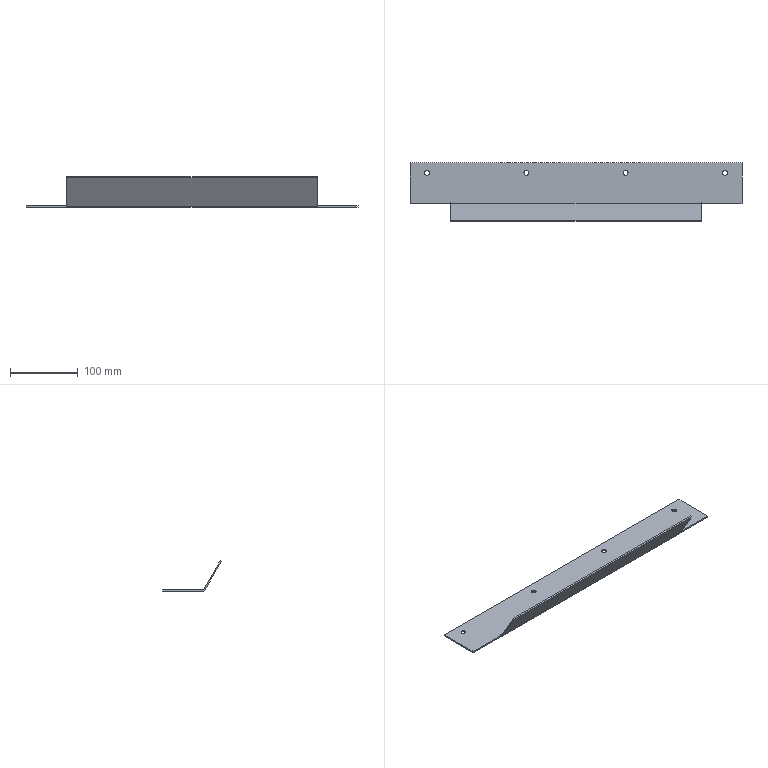Part | STEP file | zzf001 | 1 solid | 28 faces | box 488.4 x 86.155 x 44.301 mm | volume 95015 mm3 | cylinder 14 | plane 14 | commonest cylinder face diameters 7 x8 1 x5 5 x1
STEP:
#1=CARTESIAN_POINT('',(-47.004,16.182,-2.));
#2=VERTEX_POINT('',#1);
#3=CARTESIAN_POINT('',(-40.004,16.182,-2.));
#4=VERTEX_POINT('',#3);
#5=CARTESIAN_POINT('',(-43.504,16.182,-2.));
#6=DIRECTION('',(0.,0.,1.));
#7=DIRECTION('',(1.,0.,0.));
#8=AXIS2_PLACEMENT_3D('',#5,#6,#7);
#9=CIRCLE('',#8,3.5);
#10=EDGE_CURVE('',#2,#4,#9,.T.);
#11=ORIENTED_EDGE('',*,*,#10,.F.);
#12=CARTESIAN_POINT('',(-47.004,16.182,0.));
#13=VERTEX_POINT('',#12);
#14=CARTESIAN_POINT('',(-47.004,16.182,-10.));
#15=DIRECTION('',(0.,0.,1.));
#16=VECTOR('',#15,1000.);
#17=LINE('',#14,#16);
#18=EDGE_CURVE('',#2,#13,#17,.T.);
#19=ORIENTED_EDGE('',*,*,#18,.T.);
#20=CARTESIAN_POINT('',(-40.004,16.182,0.));
#21=VERTEX_POINT('',#20);
#22=CARTESIAN_POINT('',(-43.504,16.182,0.));
#23=DIRECTION('',(0.,0.,-1.));
#24=DIRECTION('',(1.,0.,0.));
#25=AXIS2_PLACEMENT_3D('',#22,#23,#24);
#26=CIRCLE('',#25,3.5);
#27=EDGE_CURVE('',#21,#13,#26,.T.);
#28=ORIENTED_EDGE('',*,*,#27,.F.);
#29=CARTESIAN_POINT('',(-40.004,16.182,-10.));
#30=DIRECTION('',(0.,0.,1.));
#31=VECTOR('',#30,1000.);
#32=LINE('',#29,#31);
#33=EDGE_CURVE('',#4,#21,#32,.T.);
#34=ORIENTED_EDGE('',*,*,#33,.F.);
#35=EDGE_LOOP('',(#11,#19,#28,#34));
#36=FACE_OUTER_BOUND('',#35,.T.);
#37=CARTESIAN_POINT('',(-43.504,16.182,-10.));
#38=DIRECTION('',(0.,0.,1.));
#39=DIRECTION('',(1.,0.,0.));
#40=AXIS2_PLACEMENT_3D('',#37,#38,#39);
#41=CYLINDRICAL_SURFACE('',#40,3.5);
#42=ADVANCED_FACE('',(#36),#41,.F.);
#43=CARTESIAN_POINT('',(99.13,16.182,-2.));
#44=VERTEX_POINT('',#43);
#45=CARTESIAN_POINT('',(106.13,16.182,-2.));
#46=VERTEX_POINT('',#45);
#47=CARTESIAN_POINT('',(102.63,16.182,-2.));
#48=DIRECTION('',(0.,0.,1.));
#49=DIRECTION('',(1.,0.,0.));
#50=AXIS2_PLACEMENT_3D('',#47,#48,#49);
#51=CIRCLE('',#50,3.5);
#52=EDGE_CURVE('',#44,#46,#51,.T.);
#53=ORIENTED_EDGE('',*,*,#52,.F.);
#54=CARTESIAN_POINT('',(99.13,16.182,0.));
#55=VERTEX_POINT('',#54);
#56=CARTESIAN_POINT('',(99.13,16.182,-10.));
#57=DIRECTION('',(0.,0.,1.));
#58=VECTOR('',#57,1000.);
#59=LINE('',#56,#58);
#60=EDGE_CURVE('',#44,#55,#59,.T.);
#61=ORIENTED_EDGE('',*,*,#60,.T.);
#62=CARTESIAN_POINT('',(106.13,16.182,0.));
#63=VERTEX_POINT('',#62);
#64=CARTESIAN_POINT('',(102.63,16.182,0.));
#65=DIRECTION('',(0.,0.,-1.));
#66=DIRECTION('',(1.,0.,0.));
#67=AXIS2_PLACEMENT_3D('',#64,#65,#66);
#68=CIRCLE('',#67,3.5);
#69=EDGE_CURVE('',#63,#55,#68,.T.);
#70=ORIENTED_EDGE('',*,*,#69,.F.);
#71=CARTESIAN_POINT('',(106.13,16.182,-10.));
#72=DIRECTION('',(0.,0.,1.));
#73=VECTOR('',#72,1000.);
#74=LINE('',#71,#73);
#75=EDGE_CURVE('',#46,#63,#74,.T.);
#76=ORIENTED_EDGE('',*,*,#75,.F.);
#77=EDGE_LOOP('',(#53,#61,#70,#76));
#78=FACE_OUTER_BOUND('',#77,.T.);
#79=CARTESIAN_POINT('',(102.63,16.182,-10.));
#80=DIRECTION('',(0.,0.,1.));
#81=DIRECTION('',(1.,0.,0.));
#82=AXIS2_PLACEMENT_3D('',#79,#80,#81);
#83=CYLINDRICAL_SURFACE('',#82,3.5);
#84=ADVANCED_FACE('',(#78),#83,.F.);
#85=CARTESIAN_POINT('',(245.263,16.182,-2.));
#86=VERTEX_POINT('',#85);
#87=CARTESIAN_POINT('',(252.263,16.182,-2.));
#88=VERTEX_POINT('',#87);
#89=CARTESIAN_POINT('',(248.763,16.182,-2.));
#90=DIRECTION('',(0.,0.,1.));
#91=DIRECTION('',(1.,0.,0.));
#92=AXIS2_PLACEMENT_3D('',#89,#90,#91);
#93=CIRCLE('',#92,3.5);
#94=EDGE_CURVE('',#86,#88,#93,.T.);
#95=ORIENTED_EDGE('',*,*,#94,.F.);
#96=CARTESIAN_POINT('',(245.263,16.182,0.));
#97=VERTEX_POINT('',#96);
#98=CARTESIAN_POINT('',(245.263,16.182,-10.));
#99=DIRECTION('',(0.,0.,1.));
#100=VECTOR('',#99,1000.);
#101=LINE('',#98,#100);
#102=EDGE_CURVE('',#86,#97,#101,.T.);
#103=ORIENTED_EDGE('',*,*,#102,.T.);
#104=CARTESIAN_POINT('',(252.263,16.182,0.));
#105=VERTEX_POINT('',#104);
#106=CARTESIAN_POINT('',(248.763,16.182,0.));
#107=DIRECTION('',(0.,0.,-1.));
#108=DIRECTION('',(1.,0.,0.));
#109=AXIS2_PLACEMENT_3D('',#106,#107,#108);
#110=CIRCLE('',#109,3.5);
#111=EDGE_CURVE('',#105,#97,#110,.T.);
#112=ORIENTED_EDGE('',*,*,#111,.F.);
#113=CARTESIAN_POINT('',(252.263,16.182,-10.));
#114=DIRECTION('',(0.,0.,1.));
#115=VECTOR('',#114,1000.);
#116=LINE('',#113,#115);
#117=EDGE_CURVE('',#88,#105,#116,.T.);
#118=ORIENTED_EDGE('',*,*,#117,.F.);
#119=EDGE_LOOP('',(#95,#103,#112,#118));
#120=FACE_OUTER_BOUND('',#119,.T.);
#121=CARTESIAN_POINT('',(248.763,16.182,-10.));
#122=DIRECTION('',(0.,0.,1.));
#123=DIRECTION('',(1.,0.,0.));
#124=AXIS2_PLACEMENT_3D('',#121,#122,#123);
#125=CYLINDRICAL_SURFACE('',#124,3.5);
#126=ADVANCED_FACE('',(#120),#125,.F.);
#127=CARTESIAN_POINT('',(391.396,16.182,-2.));
#128=VERTEX_POINT('',#127);
#129=CARTESIAN_POINT('',(398.396,16.182,-2.));
#130=VERTEX_POINT('',#129);
#131=CARTESIAN_POINT('',(394.896,16.182,-2.));
#132=DIRECTION('',(0.,0.,1.));
#133=DIRECTION('',(1.,0.,0.));
#134=AXIS2_PLACEMENT_3D('',#131,#132,#133);
#135=CIRCLE('',#134,3.5);
#136=EDGE_CURVE('',#128,#130,#135,.T.);
#137=ORIENTED_EDGE('',*,*,#136,.F.);
#138=CARTESIAN_POINT('',(391.396,16.182,0.));
#139=VERTEX_POINT('',#138);
#140=CARTESIAN_POINT('',(391.396,16.182,-10.));
#141=DIRECTION('',(0.,0.,1.));
#142=VECTOR('',#141,1000.);
#143=LINE('',#140,#142);
#144=EDGE_CURVE('',#128,#139,#143,.T.);
#145=ORIENTED_EDGE('',*,*,#144,.T.);
#146=CARTESIAN_POINT('',(398.396,16.182,0.));
#147=VERTEX_POINT('',#146);
#148=CARTESIAN_POINT('',(394.896,16.182,0.));
#149=DIRECTION('',(0.,0.,-1.));
#150=DIRECTION('',(1.,0.,0.));
#151=AXIS2_PLACEMENT_3D('',#148,#149,#150);
#152=CIRCLE('',#151,3.5);
#153=EDGE_CURVE('',#147,#139,#152,.T.);
#154=ORIENTED_EDGE('',*,*,#153,.F.);
#155=CARTESIAN_POINT('',(398.396,16.182,-10.));
#156=DIRECTION('',(0.,0.,1.));
#157=VECTOR('',#156,1000.);
#158=LINE('',#155,#157);
#159=EDGE_CURVE('',#130,#147,#158,.T.);
#160=ORIENTED_EDGE('',*,*,#159,.F.);
#161=EDGE_LOOP('',(#137,#145,#154,#160));
#162=FACE_OUTER_BOUND('',#161,.T.);
#163=CARTESIAN_POINT('',(394.896,16.182,-10.));
#164=DIRECTION('',(0.,0.,1.));
#165=DIRECTION('',(1.,0.,0.));
#166=AXIS2_PLACEMENT_3D('',#163,#164,#165);
#167=CYLINDRICAL_SURFACE('',#166,3.5);
#168=ADVANCED_FACE('',(#162),#167,.F.);
#169=CARTESIAN_POINT('',(-9.004,-27.029,0.));
#170=VERTEX_POINT('',#169);
#171=CARTESIAN_POINT('',(-8.504,-27.529,0.));
#172=VERTEX_POINT('',#171);
#173=CARTESIAN_POINT('',(-9.004,-27.529,0.));
#174=DIRECTION('',(0.,0.,-1.));
#175=DIRECTION('',(0.,1.,0.));
#176=AXIS2_PLACEMENT_3D('',#173,#174,#175);
#177=CIRCLE('',#176,0.5);
#178=EDGE_CURVE('',#170,#172,#177,.T.);
#179=ORIENTED_EDGE('',*,*,#178,.F.);
#180=CARTESIAN_POINT('',(-9.004,-27.029,-2.));
#181=VERTEX_POINT('',#180);
#182=CARTESIAN_POINT('',(-9.004,-27.029,0.));
#183=DIRECTION('',(0.,0.,-1.));
#184=VECTOR('',#183,1000.);
#185=LINE('',#182,#184);
#186=EDGE_CURVE('',#170,#181,#185,.T.);
#187=ORIENTED_EDGE('',*,*,#186,.T.);
#188=CARTESIAN_POINT('',(-8.504,-27.529,-2.));
#189=VERTEX_POINT('',#188);
#190=CARTESIAN_POINT('',(-9.004,-27.529,-2.));
#191=DIRECTION('',(0.,0.,-1.));
#192=DIRECTION('',(0.,1.,0.));
#193=AXIS2_PLACEMENT_3D('',#190,#191,#192);
#194=CIRCLE('',#193,0.5);
#195=EDGE_CURVE('',#181,#189,#194,.T.);
#196=ORIENTED_EDGE('',*,*,#195,.T.);
#197=CARTESIAN_POINT('',(-8.504,-27.529,0.));
#198=DIRECTION('',(0.,0.,-1.));
#199=VECTOR('',#198,1000.);
#200=LINE('',#197,#199);
#201=EDGE_CURVE('',#172,#189,#200,.T.);
#202=ORIENTED_EDGE('',*,*,#201,.F.);
#203=EDGE_LOOP('',(#179,#187,#196,#202));
#204=FACE_OUTER_BOUND('',#203,.T.);
#205=CARTESIAN_POINT('',(-9.004,-27.529,0.));
#206=DIRECTION('',(0.,0.,-1.));
#207=DIRECTION('',(0.,1.,0.));
#208=AXIS2_PLACEMENT_3D('',#205,#206,#207);
#209=CYLINDRICAL_SURFACE('',#208,0.5);
#210=ADVANCED_FACE('',(#204),#209,.F.);
#211=CARTESIAN_POINT('',(360.396,-27.029,0.));
#212=VERTEX_POINT('',#211);
#213=CARTESIAN_POINT('',(360.896,-27.529,0.));
#214=VERTEX_POINT('',#213);
#215=CARTESIAN_POINT('',(360.396,-27.529,0.));
#216=DIRECTION('',(0.,0.,-1.));
#217=DIRECTION('',(0.,1.,0.));
#218=AXIS2_PLACEMENT_3D('',#215,#216,#217);
#219=CIRCLE('',#218,0.5);
#220=EDGE_CURVE('',#212,#214,#219,.T.);
#221=ORIENTED_EDGE('',*,*,#220,.F.);
#222=CARTESIAN_POINT('',(360.396,-27.029,-2.));
#223=VERTEX_POINT('',#222);
#224=CARTESIAN_POINT('',(360.396,-27.029,0.));
#225=DIRECTION('',(0.,0.,-1.));
#226=VECTOR('',#225,1000.);
#227=LINE('',#224,#226);
#228=EDGE_CURVE('',#212,#223,#227,.T.);
#229=ORIENTED_EDGE('',*,*,#228,.T.);
#230=CARTESIAN_POINT('',(360.896,-27.529,-2.));
#231=VERTEX_POINT('',#230);
#232=CARTESIAN_POINT('',(360.396,-27.529,-2.));
#233=DIRECTION('',(0.,0.,1.));
#234=DIRECTION('',(0.,1.,0.));
#235=AXIS2_PLACEMENT_3D('',#232,#233,#234);
#236=CIRCLE('',#235,0.5);
#237=EDGE_CURVE('',#231,#223,#236,.T.);
#238=ORIENTED_EDGE('',*,*,#237,.F.);
#239=CARTESIAN_POINT('',(360.896,-27.529,0.));
#240=DIRECTION('',(0.,0.,-1.));
#241=VECTOR('',#240,1000.);
#242=LINE('',#239,#241);
#243=EDGE_CURVE('',#214,#231,#242,.T.);
#244=ORIENTED_EDGE('',*,*,#243,.F.);
#245=EDGE_LOOP('',(#221,#229,#238,#244));
#246=FACE_OUTER_BOUND('',#245,.T.);
#247=CARTESIAN_POINT('',(360.396,-27.529,0.));
#248=DIRECTION('',(0.,0.,-1.));
#249=DIRECTION('',(0.,1.,0.));
#250=AXIS2_PLACEMENT_3D('',#247,#248,#249);
#251=CYLINDRICAL_SURFACE('',#250,0.5);
#252=ADVANCED_FACE('',(#246),#251,.F.);
#253=CARTESIAN_POINT('',(359.896,-27.529,0.));
#254=VERTEX_POINT('',#253);
#255=CARTESIAN_POINT('',(359.896,-28.529,0.));
#256=VERTEX_POINT('',#255);
#257=CARTESIAN_POINT('',(359.896,-27.529,0.));
#258=DIRECTION('',(0.,-1.,0.));
#259=VECTOR('',#258,1000.);
#260=LINE('',#257,#259);
#261=EDGE_CURVE('',#254,#256,#260,.T.);
#262=ORIENTED_EDGE('',*,*,#261,.F.);
#263=CARTESIAN_POINT('',(360.396,-27.529,0.));
#264=DIRECTION('',(0.,0.,-1.));
#265=DIRECTION('',(0.,1.,0.));
#266=AXIS2_PLACEMENT_3D('',#263,#264,#265);
#267=CIRCLE('',#266,0.5);
#268=EDGE_CURVE('',#254,#212,#267,.T.);
#269=ORIENTED_EDGE('',*,*,#268,.T.);
#270=ORIENTED_EDGE('',*,*,#220,.T.);
#271=CARTESIAN_POINT('',(360.896,-28.818,0.));
#272=VERTEX_POINT('',#271);
#273=CARTESIAN_POINT('',(360.896,-28.818,0.));
#274=DIRECTION('',(0.,1.,0.));
#275=VECTOR('',#274,1000.);
#276=LINE('',#273,#275);
#277=EDGE_CURVE('',#272,#214,#276,.T.);
#278=ORIENTED_EDGE('',*,*,#277,.F.);
#279=CARTESIAN_POINT('',(419.896,-28.818,0.));
#280=VERTEX_POINT('',#279);
#281=CARTESIAN_POINT('',(0.,-28.818,0.));
#282=DIRECTION('',(1.,0.,0.));
#283=VECTOR('',#282,1000.);
#284=LINE('',#281,#283);
#285=EDGE_CURVE('',#272,#280,#284,.T.);
#286=ORIENTED_EDGE('',*,*,#285,.T.);
#287=CARTESIAN_POINT('',(419.896,31.182,0.));
#288=VERTEX_POINT('',#287);
#289=CARTESIAN_POINT('',(419.896,0.,0.));
#290=DIRECTION('',(0.,1.,0.));
#291=VECTOR('',#290,1000.);
#292=LINE('',#289,#291);
#293=EDGE_CURVE('',#280,#288,#292,.T.);
#294=ORIENTED_EDGE('',*,*,#293,.T.);
#295=CARTESIAN_POINT('',(-68.504,31.182,0.));
#296=VERTEX_POINT('',#295);
#297=CARTESIAN_POINT('',(0.,31.182,0.));
#298=DIRECTION('',(-1.,0.,0.));
#299=VECTOR('',#298,1000.);
#300=LINE('',#297,#299);
#301=EDGE_CURVE('',#288,#296,#300,.T.);
#302=ORIENTED_EDGE('',*,*,#301,.T.);
#303=CARTESIAN_POINT('',(-68.504,-28.818,0.));
#304=VERTEX_POINT('',#303);
#305=CARTESIAN_POINT('',(-68.504,0.,0.));
#306=DIRECTION('',(0.,-1.,0.));
#307=VECTOR('',#306,1000.);
#308=LINE('',#305,#307);
#309=EDGE_CURVE('',#296,#304,#308,.T.);
#310=ORIENTED_EDGE('',*,*,#309,.T.);
#311=CARTESIAN_POINT('',(-9.504,-28.818,0.));
#312=VERTEX_POINT('',#311);
#313=CARTESIAN_POINT('',(0.,-28.818,0.));
#314=DIRECTION('',(1.,0.,0.));
#315=VECTOR('',#314,1000.);
#316=LINE('',#313,#315);
#317=EDGE_CURVE('',#304,#312,#316,.T.);
#318=ORIENTED_EDGE('',*,*,#317,.T.);
#319=CARTESIAN_POINT('',(-9.504,-27.529,0.));
#320=VERTEX_POINT('',#319);
#321=CARTESIAN_POINT('',(-9.504,-27.529,0.));
#322=DIRECTION('',(0.,-1.,0.));
#323=VECTOR('',#322,1000.);
#324=LINE('',#321,#323);
#325=EDGE_CURVE('',#320,#312,#324,.T.);
#326=ORIENTED_EDGE('',*,*,#325,.F.);
#327=CARTESIAN_POINT('',(-9.004,-27.529,0.));
#328=DIRECTION('',(0.,0.,-1.));
#329=DIRECTION('',(0.,1.,0.));
#330=AXIS2_PLACEMENT_3D('',#327,#328,#329);
#331=CIRCLE('',#330,0.5);
#332=EDGE_CURVE('',#320,#170,#331,.T.);
#333=ORIENTED_EDGE('',*,*,#332,.T.);
#334=ORIENTED_EDGE('',*,*,#178,.T.);
#335=CARTESIAN_POINT('',(-8.504,-28.529,0.));
#336=VERTEX_POINT('',#335);
#337=CARTESIAN_POINT('',(-8.504,-28.529,0.));
#338=DIRECTION('',(0.,1.,0.));
#339=VECTOR('',#338,1000.);
#340=LINE('',#337,#339);
#341=EDGE_CURVE('',#336,#172,#340,.T.);
#342=ORIENTED_EDGE('',*,*,#341,.F.);
#343=CARTESIAN_POINT('',(0.,-28.529,0.));
#344=DIRECTION('',(1.,0.,0.));
#345=VECTOR('',#344,1000.);
#346=LINE('',#343,#345);
#347=EDGE_CURVE('',#336,#256,#346,.T.);
#348=ORIENTED_EDGE('',*,*,#347,.T.);
#349=EDGE_LOOP('',(#262,#269,#270,#278,#286,#294,#302,#310,#318,#326,#333,#334,#342,#348));
#350=FACE_OUTER_BOUND('',#349,.T.);
#351=ORIENTED_EDGE('',*,*,#27,.T.);
#352=CARTESIAN_POINT('',(-43.504,16.182,0.));
#353=DIRECTION('',(0.,0.,-1.));
#354=DIRECTION('',(1.,0.,0.));
#355=AXIS2_PLACEMENT_3D('',#352,#353,#354);
#356=CIRCLE('',#355,3.5);
#357=EDGE_CURVE('',#13,#21,#356,.T.);
#358=ORIENTED_EDGE('',*,*,#357,.T.);
#359=EDGE_LOOP('',(#351,#358));
#360=FACE_BOUND('',#359,.T.);
#361=ORIENTED_EDGE('',*,*,#69,.T.);
#362=CARTESIAN_POINT('',(102.63,16.182,0.));
#363=DIRECTION('',(0.,0.,-1.));
#364=DIRECTION('',(1.,0.,0.));
#365=AXIS2_PLACEMENT_3D('',#362,#363,#364);
#366=CIRCLE('',#365,3.5);
#367=EDGE_CURVE('',#55,#63,#366,.T.);
#368=ORIENTED_EDGE('',*,*,#367,.T.);
#369=EDGE_LOOP('',(#361,#368));
#370=FACE_BOUND('',#369,.T.);
#371=ORIENTED_EDGE('',*,*,#111,.T.);
#372=CARTESIAN_POINT('',(248.763,16.182,0.));
#373=DIRECTION('',(0.,0.,-1.));
#374=DIRECTION('',(1.,0.,0.));
#375=AXIS2_PLACEMENT_3D('',#372,#373,#374);
#376=CIRCLE('',#375,3.5);
#377=EDGE_CURVE('',#97,#105,#376,.T.);
#378=ORIENTED_EDGE('',*,*,#377,.T.);
#379=EDGE_LOOP('',(#371,#378));
#380=FACE_BOUND('',#379,.T.);
#381=ORIENTED_EDGE('',*,*,#153,.T.);
#382=CARTESIAN_POINT('',(394.896,16.182,0.));
#383=DIRECTION('',(0.,0.,-1.));
#384=DIRECTION('',(1.,0.,0.));
#385=AXIS2_PLACEMENT_3D('',#382,#383,#384);
#386=CIRCLE('',#385,3.5);
#387=EDGE_CURVE('',#139,#147,#386,.T.);
#388=ORIENTED_EDGE('',*,*,#387,.T.);
#389=EDGE_LOOP('',(#381,#388));
#390=FACE_BOUND('',#389,.T.);
#391=CARTESIAN_POINT('',(0.,0.,0.));
#392=DIRECTION('',(0.,0.,1.));
#393=DIRECTION('',(1.,0.,0.));
#394=AXIS2_PLACEMENT_3D('',#391,#392,#393);
#395=PLANE('',#394);
#396=ADVANCED_FACE('',(#350,#360,#370,#380,#390),#395,.T.);
#397=CARTESIAN_POINT('',(-8.504,-28.962,0.25));
#398=VERTEX_POINT('',#397);
#399=CARTESIAN_POINT('',(-8.504,-28.529,0.5));
#400=DIRECTION('',(1.,0.,0.));
#401=DIRECTION('',(0.,0.,-1.));
#402=AXIS2_PLACEMENT_3D('',#399,#400,#401);
#403=CIRCLE('',#402,0.5);
#404=EDGE_CURVE('',#398,#336,#403,.T.);
#405=ORIENTED_EDGE('',*,*,#404,.F.);
#406=CARTESIAN_POINT('',(359.896,-28.962,0.25));
#407=VERTEX_POINT('',#406);
#408=CARTESIAN_POINT('',(359.896,-28.962,0.25));
#409=DIRECTION('',(-1.,0.,0.));
#410=VECTOR('',#409,1000.);
#411=LINE('',#408,#410);
#412=EDGE_CURVE('',#407,#398,#411,.T.);
#413=ORIENTED_EDGE('',*,*,#412,.F.);
#414=CARTESIAN_POINT('',(359.896,-28.529,0.5));
#415=DIRECTION('',(1.,0.,0.));
#416=DIRECTION('',(0.,0.,-1.));
#417=AXIS2_PLACEMENT_3D('',#414,#415,#416);
#418=CIRCLE('',#417,0.5);
#419=EDGE_CURVE('',#407,#256,#418,.T.);
#420=ORIENTED_EDGE('',*,*,#419,.T.);
#421=ORIENTED_EDGE('',*,*,#347,.F.);
#422=EDGE_LOOP('',(#405,#413,#420,#421));
#423=FACE_OUTER_BOUND('',#422,.T.);
#424=CARTESIAN_POINT('',(359.896,-28.529,0.5));
#425=DIRECTION('',(1.,0.,0.));
#426=DIRECTION('',(0.,0.,-1.));
#427=AXIS2_PLACEMENT_3D('',#424,#425,#426);
#428=CYLINDRICAL_SURFACE('',#427,0.5);
#429=ADVANCED_FACE('',(#423),#428,.F.);
#430=ORIENTED_EDGE('',*,*,#317,.F.);
#431=CARTESIAN_POINT('',(-68.504,-28.818,-2.));
#432=VERTEX_POINT('',#431);
#433=CARTESIAN_POINT('',(-68.504,-28.818,-2.));
#434=DIRECTION('',(0.,0.,-1.));
#435=VECTOR('',#434,1000.);
#436=LINE('',#433,#435);
#437=EDGE_CURVE('',#304,#432,#436,.T.);
#438=ORIENTED_EDGE('',*,*,#437,.T.);
#439=CARTESIAN_POINT('',(-9.504,-28.818,-2.));
#440=VERTEX_POINT('',#439);
#441=CARTESIAN_POINT('',(-68.504,-28.818,-2.));
#442=DIRECTION('',(1.,0.,0.));
#443=VECTOR('',#442,1000.);
#444=LINE('',#441,#443);
#445=EDGE_CURVE('',#432,#440,#444,.T.);
#446=ORIENTED_EDGE('',*,*,#445,.T.);
#447=CARTESIAN_POINT('',(-9.504,-28.818,-2.));
#448=DIRECTION('',(0.,0.,1.));
#449=VECTOR('',#448,1000.);
#450=LINE('',#447,#449);
#451=EDGE_CURVE('',#440,#312,#450,.T.);
#452=ORIENTED_EDGE('',*,*,#451,.T.);
#453=EDGE_LOOP('',(#430,#438,#446,#452));
#454=FACE_OUTER_BOUND('',#453,.T.);
#455=CARTESIAN_POINT('',(-68.504,-28.818,-2.));
#456=DIRECTION('',(0.,-1.,0.));
#457=DIRECTION('',(0.,0.,-1.));
#458=AXIS2_PLACEMENT_3D('',#455,#456,#457);
#459=PLANE('',#458);
#460=ADVANCED_FACE('',(#454),#459,.T.);
#461=CARTESIAN_POINT('',(-68.504,31.182,-2.));
#462=VERTEX_POINT('',#461);
#463=CARTESIAN_POINT('',(-68.504,31.182,-2.));
#464=DIRECTION('',(0.,-1.,0.));
#465=VECTOR('',#464,1000.);
#466=LINE('',#463,#465);
#467=EDGE_CURVE('',#462,#432,#466,.T.);
#468=ORIENTED_EDGE('',*,*,#467,.T.);
#469=ORIENTED_EDGE('',*,*,#437,.F.);
#470=ORIENTED_EDGE('',*,*,#309,.F.);
#471=CARTESIAN_POINT('',(-68.504,31.182,-2.));
#472=DIRECTION('',(0.,0.,-1.));
#473=VECTOR('',#472,1000.);
#474=LINE('',#471,#473);
#475=EDGE_CURVE('',#296,#462,#474,.T.);
#476=ORIENTED_EDGE('',*,*,#475,.T.);
#477=EDGE_LOOP('',(#468,#469,#470,#476));
#478=FACE_OUTER_BOUND('',#477,.T.);
#479=CARTESIAN_POINT('',(-68.504,31.182,-2.));
#480=DIRECTION('',(-1.,0.,0.));
#481=DIRECTION('',(0.,0.,1.));
#482=AXIS2_PLACEMENT_3D('',#479,#480,#481);
#483=PLANE('',#482);
#484=ADVANCED_FACE('',(#478),#483,.T.);
#485=CARTESIAN_POINT('',(419.896,31.182,-2.));
#486=VERTEX_POINT('',#485);
#487=CARTESIAN_POINT('',(-68.504,31.182,-2.));
#488=DIRECTION('',(-1.,0.,0.));
#489=VECTOR('',#488,1000.);
#490=LINE('',#487,#489);
#491=EDGE_CURVE('',#486,#462,#490,.T.);
#492=ORIENTED_EDGE('',*,*,#491,.T.);
#493=ORIENTED_EDGE('',*,*,#475,.F.);
#494=ORIENTED_EDGE('',*,*,#301,.F.);
#495=CARTESIAN_POINT('',(419.896,31.182,-2.));
#496=DIRECTION('',(0.,0.,-1.));
#497=VECTOR('',#496,1000.);
#498=LINE('',#495,#497);
#499=EDGE_CURVE('',#288,#486,#498,.T.);
#500=ORIENTED_EDGE('',*,*,#499,.T.);
#501=EDGE_LOOP('',(#492,#493,#494,#500));
#502=FACE_OUTER_BOUND('',#501,.T.);
#503=CARTESIAN_POINT('',(-68.504,31.182,-2.));
#504=DIRECTION('',(0.,1.,0.));
#505=DIRECTION('',(0.,0.,1.));
#506=AXIS2_PLACEMENT_3D('',#503,#504,#505);
#507=PLANE('',#506);
#508=ADVANCED_FACE('',(#502),#507,.T.);
#509=CARTESIAN_POINT('',(419.896,-28.818,-2.));
#510=VERTEX_POINT('',#509);
#511=CARTESIAN_POINT('',(419.896,31.182,-2.));
#512=DIRECTION('',(0.,1.,0.));
#513=VECTOR('',#512,1000.);
#514=LINE('',#511,#513);
#515=EDGE_CURVE('',#510,#486,#514,.T.);
#516=ORIENTED_EDGE('',*,*,#515,.T.);
#517=ORIENTED_EDGE('',*,*,#499,.F.);
#518=ORIENTED_EDGE('',*,*,#293,.F.);
#519=CARTESIAN_POINT('',(419.896,-28.818,-2.));
#520=DIRECTION('',(0.,0.,-1.));
#521=VECTOR('',#520,1000.);
#522=LINE('',#519,#521);
#523=EDGE_CURVE('',#280,#510,#522,.T.);
#524=ORIENTED_EDGE('',*,*,#523,.T.);
#525=EDGE_LOOP('',(#516,#517,#518,#524));
#526=FACE_OUTER_BOUND('',#525,.T.);
#527=CARTESIAN_POINT('',(419.896,31.182,-2.));
#528=DIRECTION('',(1.,0.,0.));
#529=DIRECTION('',(0.,0.,-1.));
#530=AXIS2_PLACEMENT_3D('',#527,#528,#529);
#531=PLANE('',#530);
#532=ADVANCED_FACE('',(#526),#531,.T.);
#533=CARTESIAN_POINT('',(360.896,-28.818,-2.));
#534=VERTEX_POINT('',#533);
#535=CARTESIAN_POINT('',(-68.504,-28.818,-2.));
#536=DIRECTION('',(1.,0.,0.));
#537=VECTOR('',#536,1000.);
#538=LINE('',#535,#537);
#539=EDGE_CURVE('',#534,#510,#538,.T.);
#540=ORIENTED_EDGE('',*,*,#539,.T.);
#541=ORIENTED_EDGE('',*,*,#523,.F.);
#542=ORIENTED_EDGE('',*,*,#285,.F.);
#543=CARTESIAN_POINT('',(360.896,-28.818,-2.));
#544=DIRECTION('',(0.,0.,-1.));
#545=VECTOR('',#544,1000.);
#546=LINE('',#543,#545);
#547=EDGE_CURVE('',#272,#534,#546,.T.);
#548=ORIENTED_EDGE('',*,*,#547,.T.);
#549=EDGE_LOOP('',(#540,#541,#542,#548));
#550=FACE_OUTER_BOUND('',#549,.T.);
#551=CARTESIAN_POINT('',(-68.504,-28.818,-2.));
#552=DIRECTION('',(0.,-1.,0.));
#553=DIRECTION('',(0.,0.,-1.));
#554=AXIS2_PLACEMENT_3D('',#551,#552,#553);
#555=PLANE('',#554);
#556=ADVANCED_FACE('',(#550),#555,.T.);
#557=ORIENTED_EDGE('',*,*,#18,.F.);
#558=CARTESIAN_POINT('',(-43.504,16.182,-2.));
#559=DIRECTION('',(0.,0.,1.));
#560=DIRECTION('',(1.,0.,0.));
#561=AXIS2_PLACEMENT_3D('',#558,#559,#560);
#562=CIRCLE('',#561,3.5);
#563=EDGE_CURVE('',#4,#2,#562,.T.);
#564=ORIENTED_EDGE('',*,*,#563,.F.);
#565=ORIENTED_EDGE('',*,*,#33,.T.);
#566=ORIENTED_EDGE('',*,*,#357,.F.);
#567=EDGE_LOOP('',(#557,#564,#565,#566));
#568=FACE_OUTER_BOUND('',#567,.T.);
#569=CARTESIAN_POINT('',(-43.504,16.182,-10.));
#570=DIRECTION('',(0.,0.,1.));
#571=DIRECTION('',(1.,0.,0.));
#572=AXIS2_PLACEMENT_3D('',#569,#570,#571);
#573=CYLINDRICAL_SURFACE('',#572,3.5);
#574=ADVANCED_FACE('',(#568),#573,.F.);
#575=ORIENTED_EDGE('',*,*,#60,.F.);
#576=CARTESIAN_POINT('',(102.63,16.182,-2.));
#577=DIRECTION('',(0.,0.,1.));
#578=DIRECTION('',(1.,0.,0.));
#579=AXIS2_PLACEMENT_3D('',#576,#577,#578);
#580=CIRCLE('',#579,3.5);
#581=EDGE_CURVE('',#46,#44,#580,.T.);
#582=ORIENTED_EDGE('',*,*,#581,.F.);
#583=ORIENTED_EDGE('',*,*,#75,.T.);
#584=ORIENTED_EDGE('',*,*,#367,.F.);
#585=EDGE_LOOP('',(#575,#582,#583,#584));
#586=FACE_OUTER_BOUND('',#585,.T.);
#587=CARTESIAN_POINT('',(102.63,16.182,-10.));
#588=DIRECTION('',(0.,0.,1.));
#589=DIRECTION('',(1.,0.,0.));
#590=AXIS2_PLACEMENT_3D('',#587,#588,#589);
#591=CYLINDRICAL_SURFACE('',#590,3.5);
#592=ADVANCED_FACE('',(#586),#591,.F.);
#593=ORIENTED_EDGE('',*,*,#102,.F.);
#594=CARTESIAN_POINT('',(248.763,16.182,-2.));
#595=DIRECTION('',(0.,0.,1.));
#596=DIRECTION('',(1.,0.,0.));
#597=AXIS2_PLACEMENT_3D('',#594,#595,#596);
#598=CIRCLE('',#597,3.5);
#599=EDGE_CURVE('',#88,#86,#598,.T.);
#600=ORIENTED_EDGE('',*,*,#599,.F.);
#601=ORIENTED_EDGE('',*,*,#117,.T.);
#602=ORIENTED_EDGE('',*,*,#377,.F.);
#603=EDGE_LOOP('',(#593,#600,#601,#602));
#604=FACE_OUTER_BOUND('',#603,.T.);
#605=CARTESIAN_POINT('',(248.763,16.182,-10.));
#606=DIRECTION('',(0.,0.,1.));
#607=DIRECTION('',(1.,0.,0.));
#608=AXIS2_PLACEMENT_3D('',#605,#606,#607);
#609=CYLINDRICAL_SURFACE('',#608,3.5);
#610=ADVANCED_FACE('',(#604),#609,.F.);
#611=ORIENTED_EDGE('',*,*,#144,.F.);
#612=CARTESIAN_POINT('',(394.896,16.182,-2.));
#613=DIRECTION('',(0.,0.,1.));
#614=DIRECTION('',(1.,0.,0.));
#615=AXIS2_PLACEMENT_3D('',#612,#613,#614);
#616=CIRCLE('',#615,3.5);
#617=EDGE_CURVE('',#130,#128,#616,.T.);
#618=ORIENTED_EDGE('',*,*,#617,.F.);
#619=ORIENTED_EDGE('',*,*,#159,.T.);
#620=ORIENTED_EDGE('',*,*,#387,.F.);
#621=EDGE_LOOP('',(#611,#618,#619,#620));
#622=FACE_OUTER_BOUND('',#621,.T.);
#623=CARTESIAN_POINT('',(394.896,16.182,-10.));
#624=DIRECTION('',(0.,0.,1.));
#625=DIRECTION('',(1.,0.,0.));
#626=AXIS2_PLACEMENT_3D('',#623,#624,#625);
#627=CYLINDRICAL_SURFACE('',#626,3.5);
#628=ADVANCED_FACE('',(#622),#627,.F.);
#629=CARTESIAN_POINT('',(-8.504,-53.24,42.301));
#630=VERTEX_POINT('',#629);
#631=CARTESIAN_POINT('',(-8.504,-21.613,-12.478));
#632=DIRECTION('',(0.,-0.5,0.866));
#633=VECTOR('',#632,1000.);
#634=LINE('',#631,#633);
#635=EDGE_CURVE('',#398,#630,#634,.T.);
#636=ORIENTED_EDGE('',*,*,#635,.T.);
#637=CARTESIAN_POINT('',(359.896,-53.24,42.301));
#638=VERTEX_POINT('',#637);
#639=CARTESIAN_POINT('',(0.,-53.24,42.301));
#640=DIRECTION('',(1.,0.,0.));
#641=VECTOR('',#640,1000.);
#642=LINE('',#639,#641);
#643=EDGE_CURVE('',#630,#638,#642,.T.);
#644=ORIENTED_EDGE('',*,*,#643,.T.);
#645=CARTESIAN_POINT('',(359.896,-21.613,-12.478));
#646=DIRECTION('',(0.,0.5,-0.866));
#647=VECTOR('',#646,1000.);
#648=LINE('',#645,#647);
#649=EDGE_CURVE('',#638,#407,#648,.T.);
#650=ORIENTED_EDGE('',*,*,#649,.T.);
#651=ORIENTED_EDGE('',*,*,#412,.T.);
#652=EDGE_LOOP('',(#636,#644,#650,#651));
#653=FACE_OUTER_BOUND('',#652,.T.);
#654=CARTESIAN_POINT('',(0.,-21.613,-12.478));
#655=DIRECTION('',(0.,0.866,0.5));
#656=DIRECTION('',(0.,-0.5,0.866));
#657=AXIS2_PLACEMENT_3D('',#654,#655,#656);
#658=PLANE('',#657);
#659=ADVANCED_FACE('',(#653),#658,.T.);
#660=CARTESIAN_POINT('',(-9.504,-27.529,-2.));
#661=VERTEX_POINT('',#660);
#662=CARTESIAN_POINT('',(-9.504,-27.529,0.));
#663=DIRECTION('',(0.,0.,1.));
#664=VECTOR('',#663,1000.);
#665=LINE('',#662,#664);
#666=EDGE_CURVE('',#661,#320,#665,.T.);
#667=ORIENTED_EDGE('',*,*,#666,.T.);
#668=ORIENTED_EDGE('',*,*,#325,.T.);
#669=ORIENTED_EDGE('',*,*,#451,.F.);
#670=CARTESIAN_POINT('',(-9.504,-27.529,-2.));
#671=DIRECTION('',(0.,1.,0.));
#672=VECTOR('',#671,1000.);
#673=LINE('',#670,#672);
#674=EDGE_CURVE('',#440,#661,#673,.T.);
#675=ORIENTED_EDGE('',*,*,#674,.T.);
#676=EDGE_LOOP('',(#667,#668,#669,#675));
#677=FACE_OUTER_BOUND('',#676,.T.);
#678=CARTESIAN_POINT('',(-9.504,-27.529,0.));
#679=DIRECTION('',(1.,0.,0.));
#680=DIRECTION('',(0.,1.,0.));
#681=AXIS2_PLACEMENT_3D('',#678,#679,#680);
#682=PLANE('',#681);
#683=ADVANCED_FACE('',(#677),#682,.T.);
#684=ORIENTED_EDGE('',*,*,#237,.T.);
#685=CARTESIAN_POINT('',(359.896,-27.529,-2.));
#686=VERTEX_POINT('',#685);
#687=CARTESIAN_POINT('',(360.396,-27.529,-2.));
#688=DIRECTION('',(0.,0.,1.));
#689=DIRECTION('',(0.,1.,0.));
#690=AXIS2_PLACEMENT_3D('',#687,#688,#689);
#691=CIRCLE('',#690,0.5);
#692=EDGE_CURVE('',#223,#686,#691,.T.);
#693=ORIENTED_EDGE('',*,*,#692,.T.);
#694=CARTESIAN_POINT('',(359.896,-28.529,-2.));
#695=VERTEX_POINT('',#694);
#696=CARTESIAN_POINT('',(359.896,-27.529,-2.));
#697=DIRECTION('',(0.,1.,0.));
#698=VECTOR('',#697,1000.);
#699=LINE('',#696,#698);
#700=EDGE_CURVE('',#695,#686,#699,.T.);
#701=ORIENTED_EDGE('',*,*,#700,.F.);
#702=CARTESIAN_POINT('',(-8.504,-28.529,-2.));
#703=VERTEX_POINT('',#702);
#704=CARTESIAN_POINT('',(0.,-28.529,-2.));
#705=DIRECTION('',(1.,0.,0.));
#706=VECTOR('',#705,1000.);
#707=LINE('',#704,#706);
#708=EDGE_CURVE('',#703,#695,#707,.T.);
#709=ORIENTED_EDGE('',*,*,#708,.F.);
#710=CARTESIAN_POINT('',(-8.504,-28.529,-2.));
#711=DIRECTION('',(0.,-1.,0.));
#712=VECTOR('',#711,1000.);
#713=LINE('',#710,#712);
#714=EDGE_CURVE('',#189,#703,#713,.T.);
#715=ORIENTED_EDGE('',*,*,#714,.F.);
#716=ORIENTED_EDGE('',*,*,#195,.F.);
#717=CARTESIAN_POINT('',(-9.004,-27.529,-2.));
#718=DIRECTION('',(0.,0.,-1.));
#719=DIRECTION('',(0.,1.,0.));
#720=AXIS2_PLACEMENT_3D('',#717,#718,#719);
#721=CIRCLE('',#720,0.5);
#722=EDGE_CURVE('',#661,#181,#721,.T.);
#723=ORIENTED_EDGE('',*,*,#722,.F.);
#724=ORIENTED_EDGE('',*,*,#674,.F.);
#725=ORIENTED_EDGE('',*,*,#445,.F.);
#726=ORIENTED_EDGE('',*,*,#467,.F.);
#727=ORIENTED_EDGE('',*,*,#491,.F.);
#728=ORIENTED_EDGE('',*,*,#515,.F.);
#729=ORIENTED_EDGE('',*,*,#539,.F.);
#730=CARTESIAN_POINT('',(360.896,0.,-2.));
#731=DIRECTION('',(0.,-1.,0.));
#732=VECTOR('',#731,1000.);
#733=LINE('',#730,#732);
#734=EDGE_CURVE('',#231,#534,#733,.T.);
#735=ORIENTED_EDGE('',*,*,#734,.F.);
#736=EDGE_LOOP('',(#684,#693,#701,#709,#715,#716,#723,#724,#725,#726,#727,#728,#729,#735));
#737=FACE_OUTER_BOUND('',#736,.T.);
#738=ORIENTED_EDGE('',*,*,#563,.T.);
#739=ORIENTED_EDGE('',*,*,#10,.T.);
#740=EDGE_LOOP('',(#738,#739));
#741=FACE_BOUND('',#740,.T.);
#742=ORIENTED_EDGE('',*,*,#581,.T.);
#743=ORIENTED_EDGE('',*,*,#52,.T.);
#744=EDGE_LOOP('',(#742,#743));
#745=FACE_BOUND('',#744,.T.);
#746=ORIENTED_EDGE('',*,*,#599,.T.);
#747=ORIENTED_EDGE('',*,*,#94,.T.);
#748=EDGE_LOOP('',(#746,#747));
#749=FACE_BOUND('',#748,.T.);
#750=ORIENTED_EDGE('',*,*,#617,.T.);
#751=ORIENTED_EDGE('',*,*,#136,.T.);
#752=EDGE_LOOP('',(#750,#751));
#753=FACE_BOUND('',#752,.T.);
#754=CARTESIAN_POINT('',(0.,0.,-2.));
#755=DIRECTION('',(0.,0.,1.));
#756=DIRECTION('',(1.,0.,0.));
#757=AXIS2_PLACEMENT_3D('',#754,#755,#756);
#758=PLANE('',#757);
#759=ADVANCED_FACE('',(#737,#741,#745,#749,#753),#758,.F.);
#760=ORIENTED_EDGE('',*,*,#547,.F.);
#761=ORIENTED_EDGE('',*,*,#277,.T.);
#762=ORIENTED_EDGE('',*,*,#243,.T.);
#763=ORIENTED_EDGE('',*,*,#734,.T.);
#764=EDGE_LOOP('',(#760,#761,#762,#763));
#765=FACE_OUTER_BOUND('',#764,.T.);
#766=CARTESIAN_POINT('',(360.896,-28.818,0.));
#767=DIRECTION('',(-1.,0.,0.));
#768=DIRECTION('',(0.,0.,1.));
#769=AXIS2_PLACEMENT_3D('',#766,#767,#768);
#770=PLANE('',#769);
#771=ADVANCED_FACE('',(#765),#770,.T.);
#772=CARTESIAN_POINT('',(-8.504,-54.972,41.301));
#773=VERTEX_POINT('',#772);
#774=CARTESIAN_POINT('',(-8.504,-54.972,41.301));
#775=DIRECTION('',(0.,0.866,0.5));
#776=VECTOR('',#775,1000.);
#777=LINE('',#774,#776);
#778=EDGE_CURVE('',#773,#630,#777,.T.);
#779=ORIENTED_EDGE('',*,*,#778,.F.);
#780=CARTESIAN_POINT('',(359.896,-54.972,41.301));
#781=VERTEX_POINT('',#780);
#782=CARTESIAN_POINT('',(-8.504,-54.972,41.301));
#783=DIRECTION('',(-1.,0.,0.));
#784=VECTOR('',#783,1000.);
#785=LINE('',#782,#784);
#786=EDGE_CURVE('',#781,#773,#785,.T.);
#787=ORIENTED_EDGE('',*,*,#786,.F.);
#788=CARTESIAN_POINT('',(359.896,-54.972,41.301));
#789=DIRECTION('',(0.,-0.866,-0.5));
#790=VECTOR('',#789,1000.);
#791=LINE('',#788,#790);
#792=EDGE_CURVE('',#638,#781,#791,.T.);
#793=ORIENTED_EDGE('',*,*,#792,.F.);
#794=ORIENTED_EDGE('',*,*,#643,.F.);
#795=EDGE_LOOP('',(#779,#787,#793,#794));
#796=FACE_OUTER_BOUND('',#795,.T.);
#797=CARTESIAN_POINT('',(-8.504,-54.972,41.301));
#798=DIRECTION('',(0.,0.5,-0.866));
#799=DIRECTION('',(0.,0.866,0.5));
#800=AXIS2_PLACEMENT_3D('',#797,#798,#799);
#801=PLANE('',#800);
#802=ADVANCED_FACE('',(#796),#801,.F.);
#803=CARTESIAN_POINT('',(-8.504,-30.694,-0.75));
#804=VERTEX_POINT('',#803);
#805=CARTESIAN_POINT('',(-8.504,-54.972,41.301));
#806=DIRECTION('',(0.,0.5,-0.866));
#807=VECTOR('',#806,1000.);
#808=LINE('',#805,#807);
#809=EDGE_CURVE('',#773,#804,#808,.T.);
#810=ORIENTED_EDGE('',*,*,#809,.F.);
#811=ORIENTED_EDGE('',*,*,#778,.T.);
#812=ORIENTED_EDGE('',*,*,#635,.F.);
#813=ORIENTED_EDGE('',*,*,#404,.T.);
#814=ORIENTED_EDGE('',*,*,#341,.T.);
#815=ORIENTED_EDGE('',*,*,#201,.T.);
#816=ORIENTED_EDGE('',*,*,#714,.T.);
#817=CARTESIAN_POINT('',(-8.504,-28.529,0.5));
#818=DIRECTION('',(1.,0.,0.));
#819=DIRECTION('',(0.,0.,-1.));
#820=AXIS2_PLACEMENT_3D('',#817,#818,#819);
#821=CIRCLE('',#820,2.5);
#822=EDGE_CURVE('',#804,#703,#821,.T.);
#823=ORIENTED_EDGE('',*,*,#822,.F.);
#824=EDGE_LOOP('',(#810,#811,#812,#813,#814,#815,#816,#823));
#825=FACE_OUTER_BOUND('',#824,.T.);
#826=CARTESIAN_POINT('',(-8.504,-30.55,-1.));
#827=DIRECTION('',(1.,0.,0.));
#828=DIRECTION('',(0.,0.,-1.));
#829=AXIS2_PLACEMENT_3D('',#826,#827,#828);
#830=PLANE('',#829);
#831=ADVANCED_FACE('',(#825),#830,.F.);
#832=ORIENTED_EDGE('',*,*,#649,.F.);
#833=ORIENTED_EDGE('',*,*,#792,.T.);
#834=CARTESIAN_POINT('',(359.896,-30.694,-0.75));
#835=VERTEX_POINT('',#834);
#836=CARTESIAN_POINT('',(359.896,-30.694,-0.75));
#837=DIRECTION('',(0.,-0.5,0.866));
#838=VECTOR('',#837,1000.);
#839=LINE('',#836,#838);
#840=EDGE_CURVE('',#835,#781,#839,.T.);
#841=ORIENTED_EDGE('',*,*,#840,.F.);
#842=CARTESIAN_POINT('',(359.896,-28.529,0.5));
#843=DIRECTION('',(-1.,0.,0.));
#844=DIRECTION('',(0.,0.,-1.));
#845=AXIS2_PLACEMENT_3D('',#842,#843,#844);
#846=CIRCLE('',#845,2.5);
#847=EDGE_CURVE('',#695,#835,#846,.T.);
#848=ORIENTED_EDGE('',*,*,#847,.F.);
#849=ORIENTED_EDGE('',*,*,#700,.T.);
#850=CARTESIAN_POINT('',(359.896,-27.529,0.));
#851=DIRECTION('',(0.,0.,1.));
#852=VECTOR('',#851,1000.);
#853=LINE('',#850,#852);
#854=EDGE_CURVE('',#686,#254,#853,.T.);
#855=ORIENTED_EDGE('',*,*,#854,.T.);
#856=ORIENTED_EDGE('',*,*,#261,.T.);
#857=ORIENTED_EDGE('',*,*,#419,.F.);
#858=EDGE_LOOP('',(#832,#833,#841,#848,#849,#855,#856,#857));
#859=FACE_OUTER_BOUND('',#858,.T.);
#860=CARTESIAN_POINT('',(359.896,-54.972,41.301));
#861=DIRECTION('',(-1.,0.,0.));
#862=DIRECTION('',(0.,0.,1.));
#863=AXIS2_PLACEMENT_3D('',#860,#861,#862);
#864=PLANE('',#863);
#865=ADVANCED_FACE('',(#859),#864,.F.);
#866=ORIENTED_EDGE('',*,*,#186,.F.);
#867=ORIENTED_EDGE('',*,*,#332,.F.);
#868=ORIENTED_EDGE('',*,*,#666,.F.);
#869=ORIENTED_EDGE('',*,*,#722,.T.);
#870=EDGE_LOOP('',(#866,#867,#868,#869));
#871=FACE_OUTER_BOUND('',#870,.T.);
#872=CARTESIAN_POINT('',(-9.004,-27.529,0.));
#873=DIRECTION('',(0.,0.,-1.));
#874=DIRECTION('',(0.,1.,0.));
#875=AXIS2_PLACEMENT_3D('',#872,#873,#874);
#876=CYLINDRICAL_SURFACE('',#875,0.5);
#877=ADVANCED_FACE('',(#871),#876,.F.);
#878=CARTESIAN_POINT('',(359.896,-30.694,-0.75));
#879=DIRECTION('',(-1.,0.,0.));
#880=VECTOR('',#879,1000.);
#881=LINE('',#878,#880);
#882=EDGE_CURVE('',#835,#804,#881,.T.);
#883=ORIENTED_EDGE('',*,*,#882,.T.);
#884=ORIENTED_EDGE('',*,*,#822,.T.);
#885=ORIENTED_EDGE('',*,*,#708,.T.);
#886=ORIENTED_EDGE('',*,*,#847,.T.);
#887=EDGE_LOOP('',(#883,#884,#885,#886));
#888=FACE_OUTER_BOUND('',#887,.T.);
#889=CARTESIAN_POINT('',(359.896,-28.529,0.5));
#890=DIRECTION('',(1.,0.,0.));
#891=DIRECTION('',(0.,0.,-1.));
#892=AXIS2_PLACEMENT_3D('',#889,#890,#891);
#893=CYLINDRICAL_SURFACE('',#892,2.5);
#894=ADVANCED_FACE('',(#888),#893,.T.);
#895=ORIENTED_EDGE('',*,*,#228,.F.);
#896=ORIENTED_EDGE('',*,*,#268,.F.);
#897=ORIENTED_EDGE('',*,*,#854,.F.);
#898=ORIENTED_EDGE('',*,*,#692,.F.);
#899=EDGE_LOOP('',(#895,#896,#897,#898));
#900=FACE_OUTER_BOUND('',#899,.T.);
#901=CARTESIAN_POINT('',(360.396,-27.529,0.));
#902=DIRECTION('',(0.,0.,-1.));
#903=DIRECTION('',(0.,1.,0.));
#904=AXIS2_PLACEMENT_3D('',#901,#902,#903);
#905=CYLINDRICAL_SURFACE('',#904,0.5);
#906=ADVANCED_FACE('',(#900),#905,.F.);
#907=ORIENTED_EDGE('',*,*,#840,.T.);
#908=ORIENTED_EDGE('',*,*,#786,.T.);
#909=ORIENTED_EDGE('',*,*,#809,.T.);
#910=ORIENTED_EDGE('',*,*,#882,.F.);
#911=EDGE_LOOP('',(#907,#908,#909,#910));
#912=FACE_OUTER_BOUND('',#911,.T.);
#913=CARTESIAN_POINT('',(0.,-23.345,-13.478));
#914=DIRECTION('',(0.,0.866,0.5));
#915=DIRECTION('',(0.,-0.5,0.866));
#916=AXIS2_PLACEMENT_3D('',#913,#914,#915);
#917=PLANE('',#916);
#918=ADVANCED_FACE('',(#912),#917,.F.);
#919=CLOSED_SHELL('',(#42,#84,#126,#168,#210,#252,#396,#429,#460,#484,#508,#532,#556,#574,#592,#610,#628,#659,#683,#759,#771,#802,#831,#865,#877,#894,#906,#918));
#920=MANIFOLD_SOLID_BREP('',#919);
#921=CARTESIAN_POINT('',(0.,0.,0.));
#922=DIRECTION('',(0.,0.,1.));
#923=DIRECTION('',(1.,0.,0.));
#924=AXIS2_PLACEMENT_3D('',#921,#922,#923);
#925=(LENGTH_UNIT()NAMED_UNIT(*)SI_UNIT(.MILLI.,.METRE.));
#926=UNCERTAINTY_MEASURE_WITH_UNIT(LENGTH_MEASURE(0.00001),#925,'','');
#927=(NAMED_UNIT(*)PLANE_ANGLE_UNIT()SI_UNIT($,.RADIAN.));
#928=(NAMED_UNIT(*)SI_UNIT($,.STERADIAN.)SOLID_ANGLE_UNIT());
#929=(GEOMETRIC_REPRESENTATION_CONTEXT(3)GLOBAL_UNCERTAINTY_ASSIGNED_CONTEXT((#926))GLOBAL_UNIT_ASSIGNED_CONTEXT((#925,#927,#928))REPRESENTATION_CONTEXT('',''));
#930=ADVANCED_BREP_SHAPE_REPRESENTATION('',(#920,#924),#929);